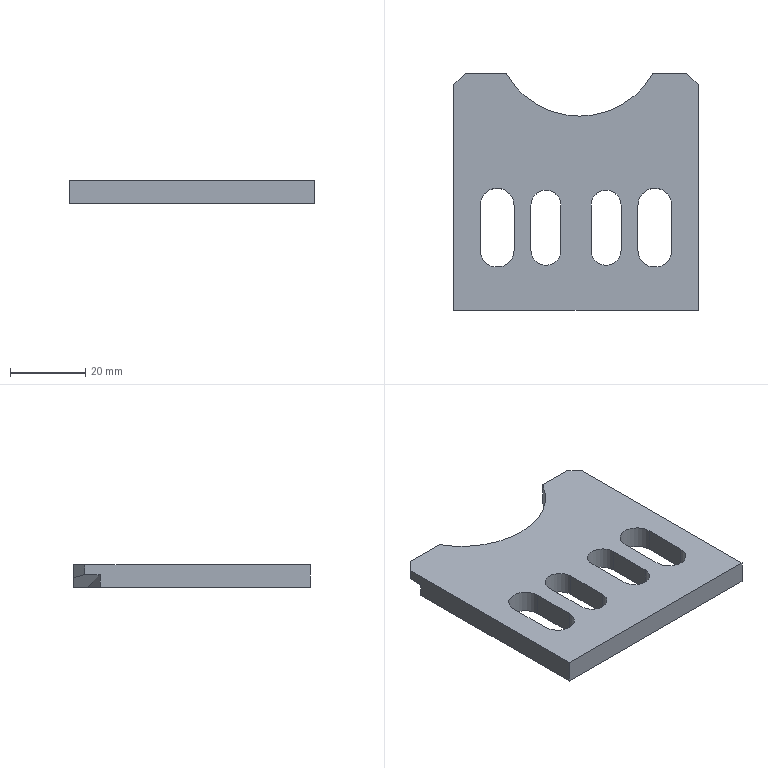Part | STEP file | gslz 2016.10.28-13_id1714_x_t | 1 solid | 31 faces | box 65 x 63 x 6 mm | volume 18675 mm3 | plane 22 | cylinder 9 | commonest cylinder face diameters 8 x4 9 x4 45 x1